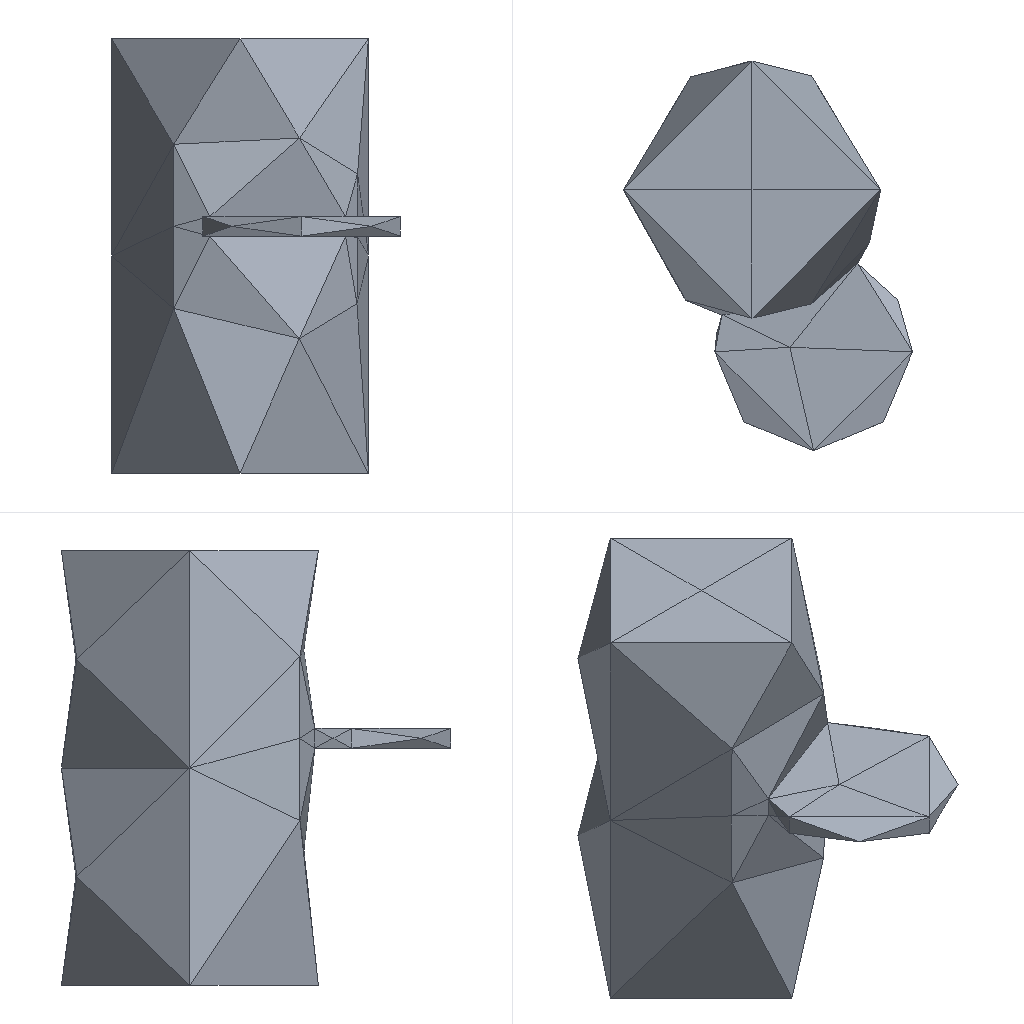Simulation study | ansys mapdl
Set-up summary:
category,name,step,type,value,unit,region
solver,ansys_mapdl
units,mm-N-s-tonne (MPa),,inferred,E=210000 density=
analysis,model,,static
mesh,nodes,,,246
mesh,elements,,,114
element_type,SOLID187,,,114
material,mat 1,,E,210000
material,mat 1,,nu,0.3
load,,model,body load temp,,,all
load,,model,force,"1000 [dir=(0, 0, -1) n=28]",,node list
bc,,model,fixed,"[dofs=UX,UY,UZ n=126]",,node list
Ansys APDL input file, long lists of numbers shortened:
/COM,ANSYS RELEASE 2026 R1           BUILD 26.1      UP20260202       09:09:22
/PREP7
/NOPR
/TITLE,2
ANTYPE, 0
*IF,_CDRDOFF,EQ,1,THEN     !if solid model was read in
_CDRDOFF=             !reset flag, numoffs already performed
*ELSE              !offset database for the following FE model
NUMOFF,NODE,      246
NUMOFF,ELEM,      114
NUMOFF,MAT ,        1
NUMOFF,TYPE,        1
*ENDIF
*SET,_RETURN ,  0.
*SET,_STATUS ,  0.
*SET,_UIQR   ,  28.
*SET,__FLOATPARAMETER__,  246.
DOF,DELETE
ETBLOCK,        1,        1
(2i9,19a9)
        1      187        0        0        0        0        0        0        0        0        0        0        0        0        0        0        0        0        0        0        0
       -1
NBLOCK,6,SOLID,       246,       246
(3i9,6e21.13e3)
        1        0        0 3.2119110472767E+001-2.6188620566304E+001 1.8000000000000E+001
! (245 more lines like these left out)
N,UNBL,LOC,       -1,
EBLOCK,19,SOLID,       114,       114
(19i10)
         1         1         1         1         0         0         0         0        10         0         1       155       159        95       160       165       166       167       168
! (227 more lines like these left out)
        -1
MPTEMP,UNBL, 1, 1,  0.    ,
MPDATA,UNBL, 1,EX  ,       1, 1,  210000.000    ,
MPTEMP,UNBL, 1, 1,  0.    ,
MPDATA,UNBL, 1,NUXY,       1, 1, 0.3    ,
MPTEMP,UNBL, 1, 1,  0.    ,
MPDATA,UNBL, 1,PRXY,       1, 1, 0.3    ,
EXTOPT,ATTR,      0,      0,      0
EXTOPT,ESIZE,  0,  0.
EXTOPT,ACLEAR,      0
TREF,  0.
IRLF,  0
BFUNIF,TEMP,_TINY
ACEL,  0.    ,  0.    ,  0.
OMEGA,  0.    ,  0.    ,  0.
DOMEGA,  0.    ,  0.    ,  0.
CGLOC,  0.    ,  0.    ,  0.
CGOMEGA,  0.    ,  0.    ,  0.
DCGOMG,  0.    ,  0.    ,  0.
KUSE,     0
TIME,  0.
ALPHAD,  0.
BETAD,  0.
DMPRAT,  0.
DMPSTR,  0.
CRPLIM, 0.1    ,   0
CRPLIM,  0.    ,   1
NCNV,     0, 1.000000000E+12,     0,  0.    ,  0.
NEQIT,     0
ERESX,DEFA
DBLOCK,       126
(i9,a6,2(pg16.9))
        8  UY    0.00000000      0.00000000
! (125 more lines like these left out)
       -1
FBLOCK,        28
(i9,a6,2(pg16.9))
       63  FZ   -35.7142857      0.00000000
! (27 more lines like these left out)
       -1
/GO
FINISH
Results summary:
result,analysis_type_db,,,static,unstated
result,n_sets,,,1,unstated
result,load_steps[0].set,load_step=1,,1,unstated
result,load_steps[0].substep,load_step=1,,1,unstated
result,load_steps[0].time,load_step=1,,1,unstated
result,load_steps[0].freq,load_step=1,,1,unstated
result,load_steps[0].max_usum,load_step=1,,0.0008562,unstated
result,load_steps[0].max_seqv,load_step=1,,12.553,unstated
result,load_steps[0].reaction_sum.FX,load_step=1,,2.413e-11,unstated
result,load_steps[0].reaction_sum.FY,load_step=1,,3.04781e-11,unstated
result,load_steps[0].reaction_sum.FZ,load_step=1,,1000,unstated
result,load_steps[0].reaction_sum.MX,load_step=1,,0,unstated
result,load_steps[0].reaction_sum.MY,load_step=1,,0,unstated
result,load_steps[0].reaction_sum.MZ,load_step=1,,0,unstated
result,convergence,,,results present for all listed sets,unstated